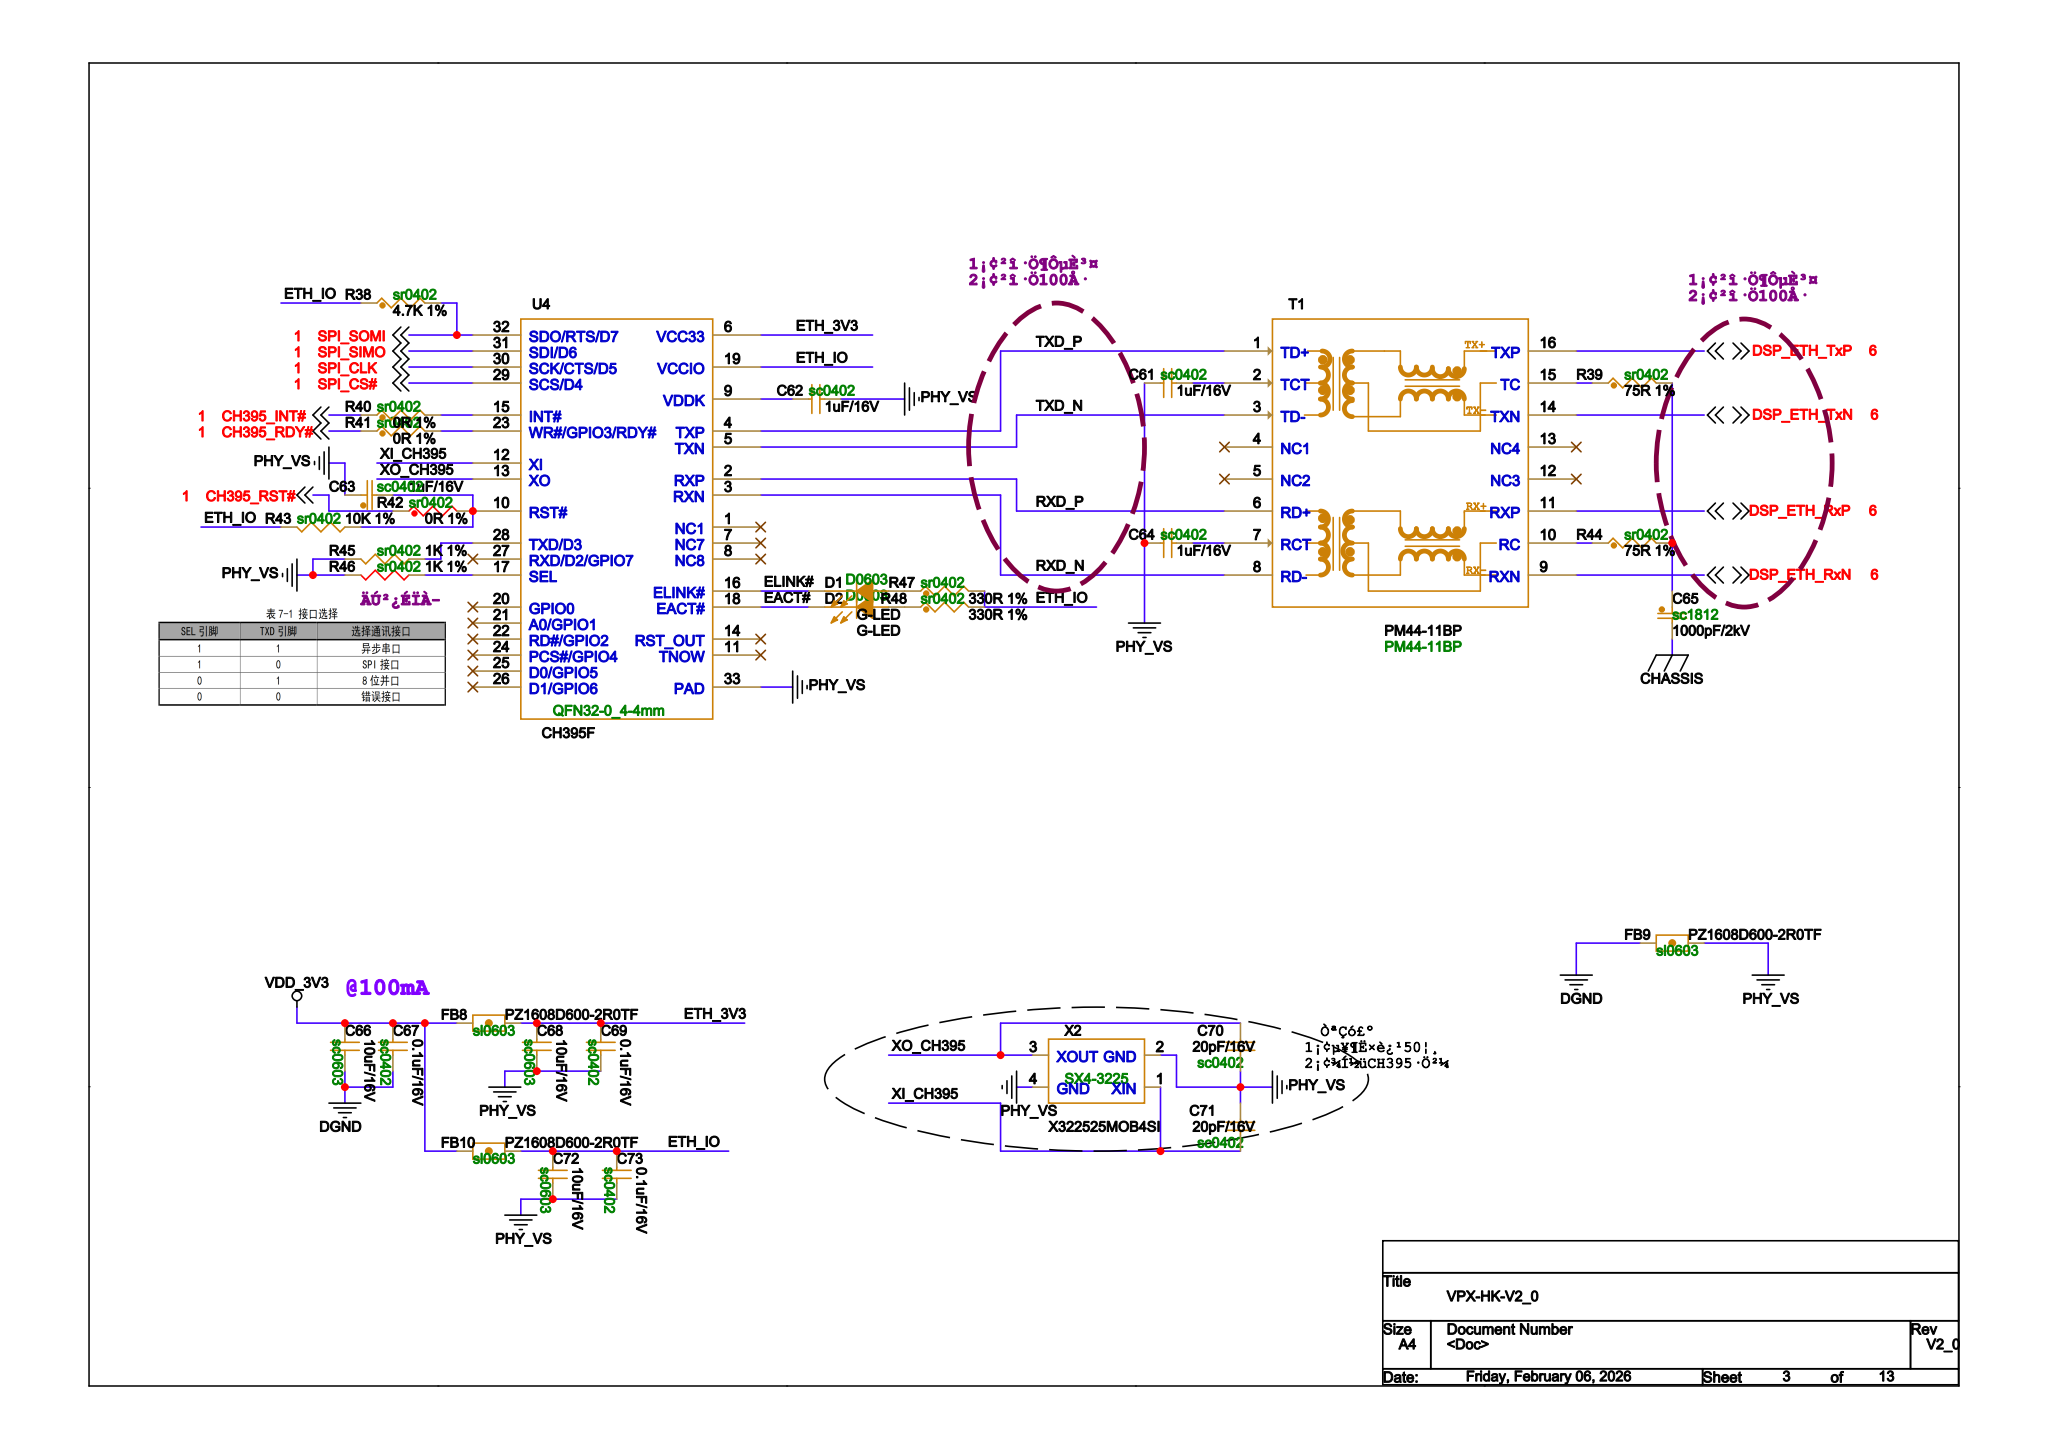Circuit board | Cadence Allegro | 598 parts | 541 nets | one sheet of the schematic
Parts on this sheet (reference | value | footprint):
C61 | 1uF/16V | SC0402
C62 | 1uF/16V | SC0402
C63 | 1uF/16V | SC0402
C64 | 1uF/16V | SC0402
C65 | 1000pF/2kV | SC1812
C70 | 20pF/16V | SC0402
C71 | 20pF/16V | SC0402
D1 | G-LED | D0603
D2 | G-LED | D0603
FB8 | PZ1608D600-2R0TF | SL0603
FB9 | PZ1608D600-2R0TF | SL0603
FB10 | PZ1608D600-2R0TF | SL0603
R38 | 4.7K 1% | SR0402
R39 | 75R 1% | SR0402
R40 | 0R 1% | SR0402
R41 | 0R 1% | SR0402
R42 | 0R 1% | SR0402
R43 | 10K 1% | SR0402
R44 | 75R 1% | SR0402
R45 | 1K 1% | SR0402
R46 | 1K 1% | SR0402
R47 | 330R 1% | SR0402
R48 | 330R 1% | SR0402
U4 | CH395F | QFN32-0_4-4MM
X2 | X322525MOB4SI | SX4-3225
Nets of these parts (net: part-pin ...):
DGND: FB9-1
CHASSIS: C65-2
VDD_3V3: FB8-1 FB10-1
ETH_IO: FB10-2 R38-1 R43-1 R47-2 R48-2 U4-19
ETH_3V3: FB8-2 U4-6
PHY_VS: C61-1 C62-2 C63-1 C64-1 C70-2 C71-1 FB9-2 R45-1 R46-1 X2-2 X2-4 U4-33
CH395_RST#: R42-1
N33628337: R45-2 U4-28
N33628602: R46-2 U4-17
N33630268: C62-1 U4-9
N33633938: C64-2
N33633918: C61-2
XI_CH395: C71-2 X2-1 U4-12
XO_CH395: C70-1 X2-3 U4-13
N33627700: C63-2 R42-2 R43-2 U4-10
SPI_SOMI: R38-2 U4-32
SPI_CLK: U4-30
SPI_CS#: U4-29
SPI_SIMO: U4-31
CH395_INT#: R40-1
CH395_RDY#: R41-1
EACT#: D2-2 U4-18
ELINK#: D1-2 U4-16
N33626531: R40-2 U4-15
RXD_N: U4-3
RXD_P: U4-2
TXD_N: U4-5
TXD_P: U4-4
N33626448: R41-2 U4-23
N336273730: D1-1 R47-1
N336273640: D2-1 R48-1
N33634330: C65-1 R39-2 R44-2
N32271831: R44-1
N32271629: R39-1